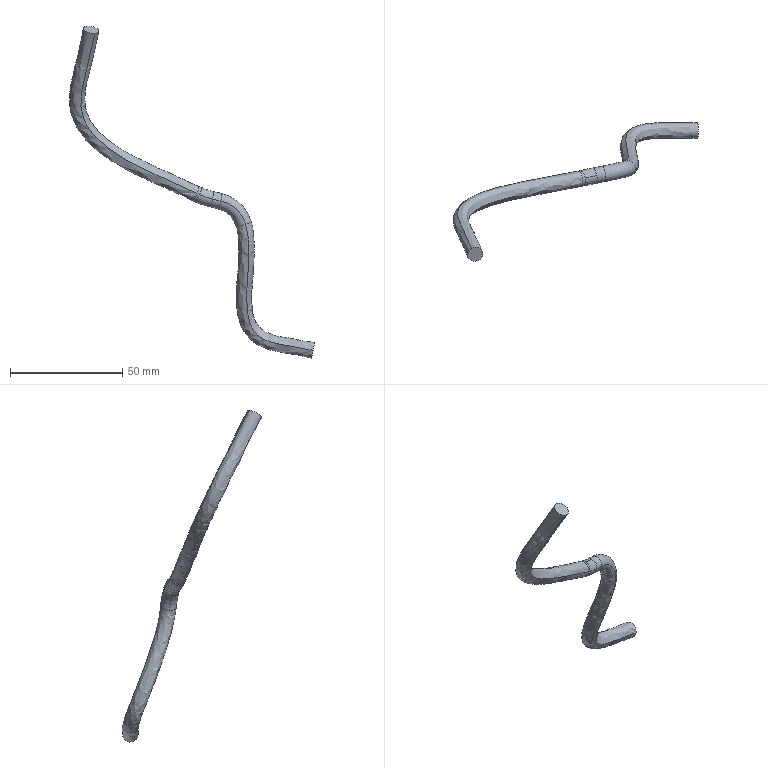Part | SolidWorks | features BaseBody 1 | 1 solid | 16 faces | box 109.447 x 62.133 x 148.234 mm | volume 8333 mm3 | torus 6 | spline 4 | cylinder 4 | plane 2 | commonest cylinder face diameters 7 x4